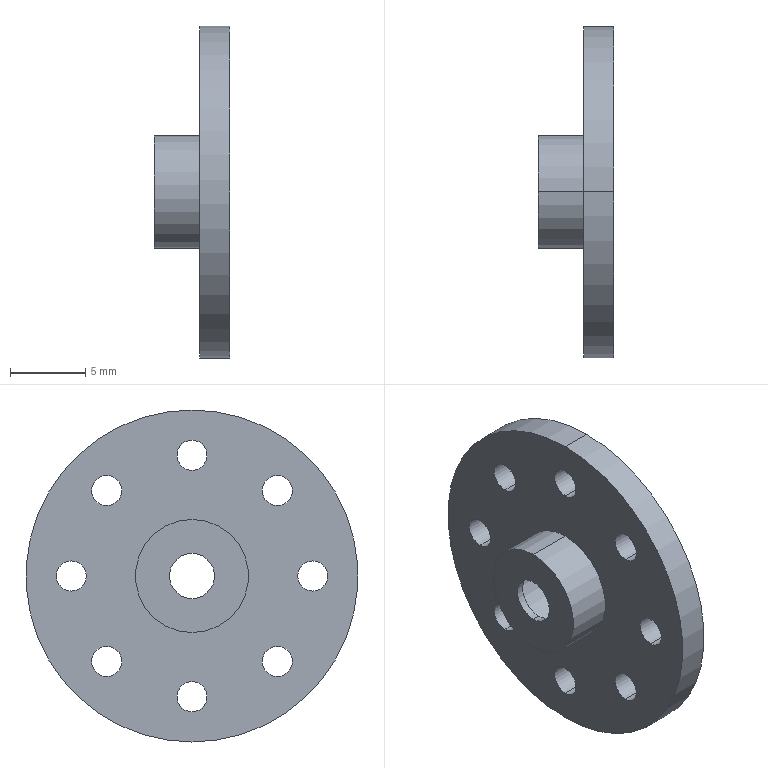Part | SolidWorks | features BaseBody 1 | 1 solid | 28 faces | box 5 x 22 x 22 mm | volume 711.767 mm3 | cylinder 24 | plane 4 | commonest cylinder face diameters 2 x16 3 x2 6 x2 7.5 x2 22 x2
STEP:
#1=CARTESIAN_POINT('',(1.,5.657,4.657));
#2=VERTEX_POINT('',#1);
#3=CARTESIAN_POINT('',(1.,5.657,6.657));
#4=VERTEX_POINT('',#3);
#5=CARTESIAN_POINT('',(1.,5.657,5.657));
#6=DIRECTION('',(-1.,0.,0.));
#7=DIRECTION('',(0.,-0.7071,0.7071));
#8=AXIS2_PLACEMENT_3D('',#5,#6,#7);
#9=CIRCLE('',#8,1.);
#10=EDGE_CURVE('',#2,#4,#9,.T.);
#11=ORIENTED_EDGE('',*,*,#10,.F.);
#12=CARTESIAN_POINT('',(-1.,5.657,4.657));
#13=VERTEX_POINT('',#12);
#14=CARTESIAN_POINT('',(1.,5.657,4.657));
#15=DIRECTION('',(-1.,0.,0.));
#16=VECTOR('',#15,1000.);
#17=LINE('',#14,#16);
#18=EDGE_CURVE('',#2,#13,#17,.T.);
#19=ORIENTED_EDGE('',*,*,#18,.T.);
#20=CARTESIAN_POINT('',(-1.,5.657,6.657));
#21=VERTEX_POINT('',#20);
#22=CARTESIAN_POINT('',(-1.,5.657,5.657));
#23=DIRECTION('',(-1.,0.,0.));
#24=DIRECTION('',(0.,-0.7071,0.7071));
#25=AXIS2_PLACEMENT_3D('',#22,#23,#24);
#26=CIRCLE('',#25,1.);
#27=EDGE_CURVE('',#13,#21,#26,.T.);
#28=ORIENTED_EDGE('',*,*,#27,.T.);
#29=CARTESIAN_POINT('',(1.,5.657,6.657));
#30=DIRECTION('',(-1.,0.,0.));
#31=VECTOR('',#30,1000.);
#32=LINE('',#29,#31);
#33=EDGE_CURVE('',#4,#21,#32,.T.);
#34=ORIENTED_EDGE('',*,*,#33,.F.);
#35=EDGE_LOOP('',(#11,#19,#28,#34));
#36=FACE_OUTER_BOUND('',#35,.T.);
#37=CARTESIAN_POINT('',(1.,5.657,5.657));
#38=DIRECTION('',(-1.,0.,0.));
#39=DIRECTION('',(0.,0.,1.));
#40=AXIS2_PLACEMENT_3D('',#37,#38,#39);
#41=CYLINDRICAL_SURFACE('',#40,1.);
#42=ADVANCED_FACE('',(#36),#41,.F.);
#43=CARTESIAN_POINT('',(1.,0.,7.));
#44=VERTEX_POINT('',#43);
#45=CARTESIAN_POINT('',(1.,0.,9.));
#46=VERTEX_POINT('',#45);
#47=CARTESIAN_POINT('',(1.,0.,8.));
#48=DIRECTION('',(-1.,0.,0.));
#49=DIRECTION('',(0.,-1.,0.));
#50=AXIS2_PLACEMENT_3D('',#47,#48,#49);
#51=CIRCLE('',#50,1.);
#52=EDGE_CURVE('',#44,#46,#51,.T.);
#53=ORIENTED_EDGE('',*,*,#52,.F.);
#54=CARTESIAN_POINT('',(-1.,0.,7.));
#55=VERTEX_POINT('',#54);
#56=CARTESIAN_POINT('',(1.,0.,7.));
#57=DIRECTION('',(-1.,0.,0.));
#58=VECTOR('',#57,1000.);
#59=LINE('',#56,#58);
#60=EDGE_CURVE('',#44,#55,#59,.T.);
#61=ORIENTED_EDGE('',*,*,#60,.T.);
#62=CARTESIAN_POINT('',(-1.,0.,9.));
#63=VERTEX_POINT('',#62);
#64=CARTESIAN_POINT('',(-1.,0.,8.));
#65=DIRECTION('',(-1.,0.,0.));
#66=DIRECTION('',(0.,-1.,0.));
#67=AXIS2_PLACEMENT_3D('',#64,#65,#66);
#68=CIRCLE('',#67,1.);
#69=EDGE_CURVE('',#55,#63,#68,.T.);
#70=ORIENTED_EDGE('',*,*,#69,.T.);
#71=CARTESIAN_POINT('',(1.,0.,9.));
#72=DIRECTION('',(-1.,0.,0.));
#73=VECTOR('',#72,1000.);
#74=LINE('',#71,#73);
#75=EDGE_CURVE('',#46,#63,#74,.T.);
#76=ORIENTED_EDGE('',*,*,#75,.F.);
#77=EDGE_LOOP('',(#53,#61,#70,#76));
#78=FACE_OUTER_BOUND('',#77,.T.);
#79=CARTESIAN_POINT('',(1.,0.,8.));
#80=DIRECTION('',(-1.,0.,0.));
#81=DIRECTION('',(0.,0.,1.));
#82=AXIS2_PLACEMENT_3D('',#79,#80,#81);
#83=CYLINDRICAL_SURFACE('',#82,1.);
#84=ADVANCED_FACE('',(#78),#83,.F.);
#85=CARTESIAN_POINT('',(1.,-5.657,4.657));
#86=VERTEX_POINT('',#85);
#87=CARTESIAN_POINT('',(1.,-5.657,6.657));
#88=VERTEX_POINT('',#87);
#89=CARTESIAN_POINT('',(1.,-5.657,5.657));
#90=DIRECTION('',(-1.,0.,0.));
#91=DIRECTION('',(0.,-0.7071,-0.7071));
#92=AXIS2_PLACEMENT_3D('',#89,#90,#91);
#93=CIRCLE('',#92,1.);
#94=EDGE_CURVE('',#86,#88,#93,.T.);
#95=ORIENTED_EDGE('',*,*,#94,.F.);
#96=CARTESIAN_POINT('',(-1.,-5.657,4.657));
#97=VERTEX_POINT('',#96);
#98=CARTESIAN_POINT('',(1.,-5.657,4.657));
#99=DIRECTION('',(-1.,0.,0.));
#100=VECTOR('',#99,1000.);
#101=LINE('',#98,#100);
#102=EDGE_CURVE('',#86,#97,#101,.T.);
#103=ORIENTED_EDGE('',*,*,#102,.T.);
#104=CARTESIAN_POINT('',(-1.,-5.657,6.657));
#105=VERTEX_POINT('',#104);
#106=CARTESIAN_POINT('',(-1.,-5.657,5.657));
#107=DIRECTION('',(-1.,0.,0.));
#108=DIRECTION('',(0.,-0.7071,-0.7071));
#109=AXIS2_PLACEMENT_3D('',#106,#107,#108);
#110=CIRCLE('',#109,1.);
#111=EDGE_CURVE('',#97,#105,#110,.T.);
#112=ORIENTED_EDGE('',*,*,#111,.T.);
#113=CARTESIAN_POINT('',(1.,-5.657,6.657));
#114=DIRECTION('',(-1.,0.,0.));
#115=VECTOR('',#114,1000.);
#116=LINE('',#113,#115);
#117=EDGE_CURVE('',#88,#105,#116,.T.);
#118=ORIENTED_EDGE('',*,*,#117,.F.);
#119=EDGE_LOOP('',(#95,#103,#112,#118));
#120=FACE_OUTER_BOUND('',#119,.T.);
#121=CARTESIAN_POINT('',(1.,-5.657,5.657));
#122=DIRECTION('',(-1.,0.,0.));
#123=DIRECTION('',(0.,0.,1.));
#124=AXIS2_PLACEMENT_3D('',#121,#122,#123);
#125=CYLINDRICAL_SURFACE('',#124,1.);
#126=ADVANCED_FACE('',(#120),#125,.F.);
#127=CARTESIAN_POINT('',(1.,-8.,-1.));
#128=VERTEX_POINT('',#127);
#129=CARTESIAN_POINT('',(1.,-8.,1.));
#130=VERTEX_POINT('',#129);
#131=CARTESIAN_POINT('',(1.,-8.,0.));
#132=DIRECTION('',(-1.,0.,0.));
#133=DIRECTION('',(0.,0.,-1.));
#134=AXIS2_PLACEMENT_3D('',#131,#132,#133);
#135=CIRCLE('',#134,1.);
#136=EDGE_CURVE('',#128,#130,#135,.T.);
#137=ORIENTED_EDGE('',*,*,#136,.F.);
#138=CARTESIAN_POINT('',(-1.,-8.,-1.));
#139=VERTEX_POINT('',#138);
#140=CARTESIAN_POINT('',(1.,-8.,-1.));
#141=DIRECTION('',(-1.,0.,0.));
#142=VECTOR('',#141,1000.);
#143=LINE('',#140,#142);
#144=EDGE_CURVE('',#128,#139,#143,.T.);
#145=ORIENTED_EDGE('',*,*,#144,.T.);
#146=CARTESIAN_POINT('',(-1.,-8.,1.));
#147=VERTEX_POINT('',#146);
#148=CARTESIAN_POINT('',(-1.,-8.,0.));
#149=DIRECTION('',(-1.,0.,0.));
#150=DIRECTION('',(0.,0.,-1.));
#151=AXIS2_PLACEMENT_3D('',#148,#149,#150);
#152=CIRCLE('',#151,1.);
#153=EDGE_CURVE('',#139,#147,#152,.T.);
#154=ORIENTED_EDGE('',*,*,#153,.T.);
#155=CARTESIAN_POINT('',(1.,-8.,1.));
#156=DIRECTION('',(-1.,0.,0.));
#157=VECTOR('',#156,1000.);
#158=LINE('',#155,#157);
#159=EDGE_CURVE('',#130,#147,#158,.T.);
#160=ORIENTED_EDGE('',*,*,#159,.F.);
#161=EDGE_LOOP('',(#137,#145,#154,#160));
#162=FACE_OUTER_BOUND('',#161,.T.);
#163=CARTESIAN_POINT('',(1.,-8.,0.));
#164=DIRECTION('',(-1.,0.,0.));
#165=DIRECTION('',(0.,0.,1.));
#166=AXIS2_PLACEMENT_3D('',#163,#164,#165);
#167=CYLINDRICAL_SURFACE('',#166,1.);
#168=ADVANCED_FACE('',(#162),#167,.F.);
#169=CARTESIAN_POINT('',(1.,-5.657,-6.657));
#170=VERTEX_POINT('',#169);
#171=CARTESIAN_POINT('',(1.,-5.657,-4.657));
#172=VERTEX_POINT('',#171);
#173=CARTESIAN_POINT('',(1.,-5.657,-5.657));
#174=DIRECTION('',(-1.,0.,0.));
#175=DIRECTION('',(0.,0.7071,-0.7071));
#176=AXIS2_PLACEMENT_3D('',#173,#174,#175);
#177=CIRCLE('',#176,1.);
#178=EDGE_CURVE('',#170,#172,#177,.T.);
#179=ORIENTED_EDGE('',*,*,#178,.F.);
#180=CARTESIAN_POINT('',(-1.,-5.657,-6.657));
#181=VERTEX_POINT('',#180);
#182=CARTESIAN_POINT('',(1.,-5.657,-6.657));
#183=DIRECTION('',(-1.,0.,0.));
#184=VECTOR('',#183,1000.);
#185=LINE('',#182,#184);
#186=EDGE_CURVE('',#170,#181,#185,.T.);
#187=ORIENTED_EDGE('',*,*,#186,.T.);
#188=CARTESIAN_POINT('',(-1.,-5.657,-4.657));
#189=VERTEX_POINT('',#188);
#190=CARTESIAN_POINT('',(-1.,-5.657,-5.657));
#191=DIRECTION('',(-1.,0.,0.));
#192=DIRECTION('',(0.,0.7071,-0.7071));
#193=AXIS2_PLACEMENT_3D('',#190,#191,#192);
#194=CIRCLE('',#193,1.);
#195=EDGE_CURVE('',#181,#189,#194,.T.);
#196=ORIENTED_EDGE('',*,*,#195,.T.);
#197=CARTESIAN_POINT('',(1.,-5.657,-4.657));
#198=DIRECTION('',(-1.,0.,0.));
#199=VECTOR('',#198,1000.);
#200=LINE('',#197,#199);
#201=EDGE_CURVE('',#172,#189,#200,.T.);
#202=ORIENTED_EDGE('',*,*,#201,.F.);
#203=EDGE_LOOP('',(#179,#187,#196,#202));
#204=FACE_OUTER_BOUND('',#203,.T.);
#205=CARTESIAN_POINT('',(1.,-5.657,-5.657));
#206=DIRECTION('',(-1.,0.,0.));
#207=DIRECTION('',(0.,0.,1.));
#208=AXIS2_PLACEMENT_3D('',#205,#206,#207);
#209=CYLINDRICAL_SURFACE('',#208,1.);
#210=ADVANCED_FACE('',(#204),#209,.F.);
#211=CARTESIAN_POINT('',(1.,0.,-9.));
#212=VERTEX_POINT('',#211);
#213=CARTESIAN_POINT('',(1.,0.,-7.));
#214=VERTEX_POINT('',#213);
#215=CARTESIAN_POINT('',(1.,0.,-8.));
#216=DIRECTION('',(-1.,0.,0.));
#217=DIRECTION('',(0.,1.,0.));
#218=AXIS2_PLACEMENT_3D('',#215,#216,#217);
#219=CIRCLE('',#218,1.);
#220=EDGE_CURVE('',#212,#214,#219,.T.);
#221=ORIENTED_EDGE('',*,*,#220,.F.);
#222=CARTESIAN_POINT('',(-1.,0.,-9.));
#223=VERTEX_POINT('',#222);
#224=CARTESIAN_POINT('',(1.,0.,-9.));
#225=DIRECTION('',(-1.,0.,0.));
#226=VECTOR('',#225,1000.);
#227=LINE('',#224,#226);
#228=EDGE_CURVE('',#212,#223,#227,.T.);
#229=ORIENTED_EDGE('',*,*,#228,.T.);
#230=CARTESIAN_POINT('',(-1.,0.,-7.));
#231=VERTEX_POINT('',#230);
#232=CARTESIAN_POINT('',(-1.,0.,-8.));
#233=DIRECTION('',(-1.,0.,0.));
#234=DIRECTION('',(0.,1.,0.));
#235=AXIS2_PLACEMENT_3D('',#232,#233,#234);
#236=CIRCLE('',#235,1.);
#237=EDGE_CURVE('',#223,#231,#236,.T.);
#238=ORIENTED_EDGE('',*,*,#237,.T.);
#239=CARTESIAN_POINT('',(1.,0.,-7.));
#240=DIRECTION('',(-1.,0.,0.));
#241=VECTOR('',#240,1000.);
#242=LINE('',#239,#241);
#243=EDGE_CURVE('',#214,#231,#242,.T.);
#244=ORIENTED_EDGE('',*,*,#243,.F.);
#245=EDGE_LOOP('',(#221,#229,#238,#244));
#246=FACE_OUTER_BOUND('',#245,.T.);
#247=CARTESIAN_POINT('',(1.,0.,-8.));
#248=DIRECTION('',(-1.,0.,0.));
#249=DIRECTION('',(0.,0.,1.));
#250=AXIS2_PLACEMENT_3D('',#247,#248,#249);
#251=CYLINDRICAL_SURFACE('',#250,1.);
#252=ADVANCED_FACE('',(#246),#251,.F.);
#253=CARTESIAN_POINT('',(1.,5.657,-6.657));
#254=VERTEX_POINT('',#253);
#255=CARTESIAN_POINT('',(1.,5.657,-4.657));
#256=VERTEX_POINT('',#255);
#257=CARTESIAN_POINT('',(1.,5.657,-5.657));
#258=DIRECTION('',(-1.,0.,0.));
#259=DIRECTION('',(0.,0.7071,0.7071));
#260=AXIS2_PLACEMENT_3D('',#257,#258,#259);
#261=CIRCLE('',#260,1.);
#262=EDGE_CURVE('',#254,#256,#261,.T.);
#263=ORIENTED_EDGE('',*,*,#262,.F.);
#264=CARTESIAN_POINT('',(-1.,5.657,-6.657));
#265=VERTEX_POINT('',#264);
#266=CARTESIAN_POINT('',(1.,5.657,-6.657));
#267=DIRECTION('',(-1.,0.,0.));
#268=VECTOR('',#267,1000.);
#269=LINE('',#266,#268);
#270=EDGE_CURVE('',#254,#265,#269,.T.);
#271=ORIENTED_EDGE('',*,*,#270,.T.);
#272=CARTESIAN_POINT('',(-1.,5.657,-4.657));
#273=VERTEX_POINT('',#272);
#274=CARTESIAN_POINT('',(-1.,5.657,-5.657));
#275=DIRECTION('',(-1.,0.,0.));
#276=DIRECTION('',(0.,0.7071,0.7071));
#277=AXIS2_PLACEMENT_3D('',#274,#275,#276);
#278=CIRCLE('',#277,1.);
#279=EDGE_CURVE('',#265,#273,#278,.T.);
#280=ORIENTED_EDGE('',*,*,#279,.T.);
#281=CARTESIAN_POINT('',(1.,5.657,-4.657));
#282=DIRECTION('',(-1.,0.,0.));
#283=VECTOR('',#282,1000.);
#284=LINE('',#281,#283);
#285=EDGE_CURVE('',#256,#273,#284,.T.);
#286=ORIENTED_EDGE('',*,*,#285,.F.);
#287=EDGE_LOOP('',(#263,#271,#280,#286));
#288=FACE_OUTER_BOUND('',#287,.T.);
#289=CARTESIAN_POINT('',(1.,5.657,-5.657));
#290=DIRECTION('',(-1.,0.,0.));
#291=DIRECTION('',(0.,0.,1.));
#292=AXIS2_PLACEMENT_3D('',#289,#290,#291);
#293=CYLINDRICAL_SURFACE('',#292,1.);
#294=ADVANCED_FACE('',(#288),#293,.F.);
#295=CARTESIAN_POINT('',(1.,8.,-1.));
#296=VERTEX_POINT('',#295);
#297=CARTESIAN_POINT('',(1.,8.,1.));
#298=VERTEX_POINT('',#297);
#299=CARTESIAN_POINT('',(1.,8.,0.));
#300=DIRECTION('',(-1.,0.,0.));
#301=DIRECTION('',(0.,0.,1.));
#302=AXIS2_PLACEMENT_3D('',#299,#300,#301);
#303=CIRCLE('',#302,1.);
#304=EDGE_CURVE('',#296,#298,#303,.T.);
#305=ORIENTED_EDGE('',*,*,#304,.F.);
#306=CARTESIAN_POINT('',(-1.,8.,-1.));
#307=VERTEX_POINT('',#306);
#308=CARTESIAN_POINT('',(1.,8.,-1.));
#309=DIRECTION('',(-1.,0.,0.));
#310=VECTOR('',#309,1000.);
#311=LINE('',#308,#310);
#312=EDGE_CURVE('',#296,#307,#311,.T.);
#313=ORIENTED_EDGE('',*,*,#312,.T.);
#314=CARTESIAN_POINT('',(-1.,8.,1.));
#315=VERTEX_POINT('',#314);
#316=CARTESIAN_POINT('',(-1.,8.,0.));
#317=DIRECTION('',(-1.,0.,0.));
#318=DIRECTION('',(0.,0.,1.));
#319=AXIS2_PLACEMENT_3D('',#316,#317,#318);
#320=CIRCLE('',#319,1.);
#321=EDGE_CURVE('',#307,#315,#320,.T.);
#322=ORIENTED_EDGE('',*,*,#321,.T.);
#323=CARTESIAN_POINT('',(1.,8.,1.));
#324=DIRECTION('',(-1.,0.,0.));
#325=VECTOR('',#324,1000.);
#326=LINE('',#323,#325);
#327=EDGE_CURVE('',#298,#315,#326,.T.);
#328=ORIENTED_EDGE('',*,*,#327,.F.);
#329=EDGE_LOOP('',(#305,#313,#322,#328));
#330=FACE_OUTER_BOUND('',#329,.T.);
#331=CARTESIAN_POINT('',(1.,8.,0.));
#332=DIRECTION('',(-1.,0.,0.));
#333=DIRECTION('',(0.,0.,1.));
#334=AXIS2_PLACEMENT_3D('',#331,#332,#333);
#335=CYLINDRICAL_SURFACE('',#334,1.);
#336=ADVANCED_FACE('',(#330),#335,.F.);
#337=CARTESIAN_POINT('',(1.,0.,-3.));
#338=VERTEX_POINT('',#337);
#339=CARTESIAN_POINT('',(1.,0.,3.));
#340=VERTEX_POINT('',#339);
#341=CARTESIAN_POINT('',(1.,0.,0.));
#342=DIRECTION('',(-1.,0.,0.));
#343=DIRECTION('',(0.,0.,1.));
#344=AXIS2_PLACEMENT_3D('',#341,#342,#343);
#345=CIRCLE('',#344,3.);
#346=EDGE_CURVE('',#338,#340,#345,.T.);
#347=ORIENTED_EDGE('',*,*,#346,.F.);
#348=CARTESIAN_POINT('',(-3.5,0.,-3.));
#349=VERTEX_POINT('',#348);
#350=CARTESIAN_POINT('',(0.,0.,-3.));
#351=DIRECTION('',(-1.,0.,0.));
#352=VECTOR('',#351,1000.);
#353=LINE('',#350,#352);
#354=EDGE_CURVE('',#338,#349,#353,.T.);
#355=ORIENTED_EDGE('',*,*,#354,.T.);
#356=CARTESIAN_POINT('',(-3.5,0.,3.));
#357=VERTEX_POINT('',#356);
#358=CARTESIAN_POINT('',(-3.5,0.,0.));
#359=DIRECTION('',(-1.,0.,0.));
#360=DIRECTION('',(0.,0.,1.));
#361=AXIS2_PLACEMENT_3D('',#358,#359,#360);
#362=CIRCLE('',#361,3.);
#363=EDGE_CURVE('',#349,#357,#362,.T.);
#364=ORIENTED_EDGE('',*,*,#363,.T.);
#365=CARTESIAN_POINT('',(0.,0.,3.));
#366=DIRECTION('',(-1.,0.,0.));
#367=VECTOR('',#366,1000.);
#368=LINE('',#365,#367);
#369=EDGE_CURVE('',#340,#357,#368,.T.);
#370=ORIENTED_EDGE('',*,*,#369,.F.);
#371=EDGE_LOOP('',(#347,#355,#364,#370));
#372=FACE_OUTER_BOUND('',#371,.T.);
#373=CARTESIAN_POINT('',(0.,0.,0.));
#374=DIRECTION('',(-1.,0.,0.));
#375=DIRECTION('',(0.,0.,1.));
#376=AXIS2_PLACEMENT_3D('',#373,#374,#375);
#377=CYLINDRICAL_SURFACE('',#376,3.);
#378=ADVANCED_FACE('',(#372),#377,.F.);
#379=CARTESIAN_POINT('',(-3.5,0.,-1.5));
#380=VERTEX_POINT('',#379);
#381=CARTESIAN_POINT('',(-3.5,0.,1.5));
#382=VERTEX_POINT('',#381);
#383=CARTESIAN_POINT('',(-3.5,0.,0.));
#384=DIRECTION('',(-1.,0.,0.));
#385=DIRECTION('',(0.,0.,1.));
#386=AXIS2_PLACEMENT_3D('',#383,#384,#385);
#387=CIRCLE('',#386,1.5);
#388=EDGE_CURVE('',#380,#382,#387,.T.);
#389=ORIENTED_EDGE('',*,*,#388,.F.);
#390=CARTESIAN_POINT('',(-4.,0.,-1.5));
#391=VERTEX_POINT('',#390);
#392=CARTESIAN_POINT('',(0.,0.,-1.5));
#393=DIRECTION('',(-1.,0.,0.));
#394=VECTOR('',#393,1000.);
#395=LINE('',#392,#394);
#396=EDGE_CURVE('',#380,#391,#395,.T.);
#397=ORIENTED_EDGE('',*,*,#396,.T.);
#398=CARTESIAN_POINT('',(-4.,0.,1.5));
#399=VERTEX_POINT('',#398);
#400=CARTESIAN_POINT('',(-4.,0.,0.));
#401=DIRECTION('',(-1.,0.,0.));
#402=DIRECTION('',(0.,0.,1.));
#403=AXIS2_PLACEMENT_3D('',#400,#401,#402);
#404=CIRCLE('',#403,1.5);
#405=EDGE_CURVE('',#391,#399,#404,.T.);
#406=ORIENTED_EDGE('',*,*,#405,.T.);
#407=CARTESIAN_POINT('',(0.,0.,1.5));
#408=DIRECTION('',(-1.,0.,0.));
#409=VECTOR('',#408,1000.);
#410=LINE('',#407,#409);
#411=EDGE_CURVE('',#382,#399,#410,.T.);
#412=ORIENTED_EDGE('',*,*,#411,.F.);
#413=EDGE_LOOP('',(#389,#397,#406,#412));
#414=FACE_OUTER_BOUND('',#413,.T.);
#415=CARTESIAN_POINT('',(0.,0.,0.));
#416=DIRECTION('',(-1.,0.,0.));
#417=DIRECTION('',(0.,0.,1.));
#418=AXIS2_PLACEMENT_3D('',#415,#416,#417);
#419=CYLINDRICAL_SURFACE('',#418,1.5);
#420=ADVANCED_FACE('',(#414),#419,.F.);
#421=CARTESIAN_POINT('',(-1.,0.,3.75));
#422=VERTEX_POINT('',#421);
#423=CARTESIAN_POINT('',(-1.,0.,-3.75));
#424=VERTEX_POINT('',#423);
#425=CARTESIAN_POINT('',(-1.,0.,0.));
#426=DIRECTION('',(-1.,0.,0.));
#427=DIRECTION('',(0.,0.,1.));
#428=AXIS2_PLACEMENT_3D('',#425,#426,#427);
#429=CIRCLE('',#428,3.75);
#430=EDGE_CURVE('',#422,#424,#429,.T.);
#431=ORIENTED_EDGE('',*,*,#430,.T.);
#432=CARTESIAN_POINT('',(-4.,0.,-3.75));
#433=VERTEX_POINT('',#432);
#434=CARTESIAN_POINT('',(0.,0.,-3.75));
#435=DIRECTION('',(-1.,0.,0.));
#436=VECTOR('',#435,1000.);
#437=LINE('',#434,#436);
#438=EDGE_CURVE('',#424,#433,#437,.T.);
#439=ORIENTED_EDGE('',*,*,#438,.T.);
#440=CARTESIAN_POINT('',(-4.,0.,3.75));
#441=VERTEX_POINT('',#440);
#442=CARTESIAN_POINT('',(-4.,0.,0.));
#443=DIRECTION('',(-1.,0.,0.));
#444=DIRECTION('',(0.,0.,1.));
#445=AXIS2_PLACEMENT_3D('',#442,#443,#444);
#446=CIRCLE('',#445,3.75);
#447=EDGE_CURVE('',#441,#433,#446,.T.);
#448=ORIENTED_EDGE('',*,*,#447,.F.);
#449=CARTESIAN_POINT('',(0.,0.,3.75));
#450=DIRECTION('',(-1.,0.,0.));
#451=VECTOR('',#450,1000.);
#452=LINE('',#449,#451);
#453=EDGE_CURVE('',#422,#441,#452,.T.);
#454=ORIENTED_EDGE('',*,*,#453,.F.);
#455=EDGE_LOOP('',(#431,#439,#448,#454));
#456=FACE_OUTER_BOUND('',#455,.T.);
#457=CARTESIAN_POINT('',(0.,0.,0.));
#458=DIRECTION('',(-1.,0.,0.));
#459=DIRECTION('',(0.,0.,1.));
#460=AXIS2_PLACEMENT_3D('',#457,#458,#459);
#461=CYLINDRICAL_SURFACE('',#460,3.75);
#462=ADVANCED_FACE('',(#456),#461,.T.);
#463=CARTESIAN_POINT('',(1.,0.,11.));
#464=VERTEX_POINT('',#463);
#465=CARTESIAN_POINT('',(1.,0.,-11.));
#466=VERTEX_POINT('',#465);
#467=CARTESIAN_POINT('',(1.,0.,0.));
#468=DIRECTION('',(-1.,0.,0.));
#469=DIRECTION('',(0.,0.,1.));
#470=AXIS2_PLACEMENT_3D('',#467,#468,#469);
#471=CIRCLE('',#470,11.);
#472=EDGE_CURVE('',#464,#466,#471,.T.);
#473=ORIENTED_EDGE('',*,*,#472,.T.);
#474=CARTESIAN_POINT('',(-1.,0.,-11.));
#475=VERTEX_POINT('',#474);
#476=CARTESIAN_POINT('',(0.,0.,-11.));
#477=DIRECTION('',(-1.,0.,0.));
#478=VECTOR('',#477,1000.);
#479=LINE('',#476,#478);
#480=EDGE_CURVE('',#466,#475,#479,.T.);
#481=ORIENTED_EDGE('',*,*,#480,.T.);
#482=CARTESIAN_POINT('',(-1.,0.,11.));
#483=VERTEX_POINT('',#482);
#484=CARTESIAN_POINT('',(-1.,0.,0.));
#485=DIRECTION('',(-1.,0.,0.));
#486=DIRECTION('',(0.,0.,1.));
#487=AXIS2_PLACEMENT_3D('',#484,#485,#486);
#488=CIRCLE('',#487,11.);
#489=EDGE_CURVE('',#483,#475,#488,.T.);
#490=ORIENTED_EDGE('',*,*,#489,.F.);
#491=CARTESIAN_POINT('',(0.,0.,11.));
#492=DIRECTION('',(-1.,0.,0.));
#493=VECTOR('',#492,1000.);
#494=LINE('',#491,#493);
#495=EDGE_CURVE('',#464,#483,#494,.T.);
#496=ORIENTED_EDGE('',*,*,#495,.F.);
#497=EDGE_LOOP('',(#473,#481,#490,#496));
#498=FACE_OUTER_BOUND('',#497,.T.);
#499=CARTESIAN_POINT('',(0.,0.,0.));
#500=DIRECTION('',(-1.,0.,0.));
#501=DIRECTION('',(0.,0.,1.));
#502=AXIS2_PLACEMENT_3D('',#499,#500,#501);
#503=CYLINDRICAL_SURFACE('',#502,11.);
#504=ADVANCED_FACE('',(#498),#503,.T.);
#505=CARTESIAN_POINT('',(1.,5.657,5.657));
#506=DIRECTION('',(-1.,0.,0.));
#507=DIRECTION('',(0.,-0.7071,0.7071));
#508=AXIS2_PLACEMENT_3D('',#505,#506,#507);
#509=CIRCLE('',#508,1.);
#510=EDGE_CURVE('',#4,#2,#509,.T.);
#511=ORIENTED_EDGE('',*,*,#510,.T.);
#512=ORIENTED_EDGE('',*,*,#10,.T.);
#513=EDGE_LOOP('',(#511,#512));
#514=FACE_BOUND('',#513,.T.);
#515=CARTESIAN_POINT('',(1.,0.,8.));
#516=DIRECTION('',(-1.,0.,0.));
#517=DIRECTION('',(0.,-1.,0.));
#518=AXIS2_PLACEMENT_3D('',#515,#516,#517);
#519=CIRCLE('',#518,1.);
#520=EDGE_CURVE('',#46,#44,#519,.T.);
#521=ORIENTED_EDGE('',*,*,#520,.T.);
#522=ORIENTED_EDGE('',*,*,#52,.T.);
#523=EDGE_LOOP('',(#521,#522));
#524=FACE_BOUND('',#523,.T.);
#525=CARTESIAN_POINT('',(1.,-5.657,5.657));
#526=DIRECTION('',(-1.,0.,0.));
#527=DIRECTION('',(0.,-0.7071,-0.7071));
#528=AXIS2_PLACEMENT_3D('',#525,#526,#527);
#529=CIRCLE('',#528,1.);
#530=EDGE_CURVE('',#88,#86,#529,.T.);
#531=ORIENTED_EDGE('',*,*,#530,.T.);
#532=ORIENTED_EDGE('',*,*,#94,.T.);
#533=EDGE_LOOP('',(#531,#532));
#534=FACE_BOUND('',#533,.T.);
#535=CARTESIAN_POINT('',(1.,-8.,0.));
#536=DIRECTION('',(-1.,0.,0.));
#537=DIRECTION('',(0.,0.,-1.));
#538=AXIS2_PLACEMENT_3D('',#535,#536,#537);
#539=CIRCLE('',#538,1.);
#540=EDGE_CURVE('',#130,#128,#539,.T.);
#541=ORIENTED_EDGE('',*,*,#540,.T.);
#542=ORIENTED_EDGE('',*,*,#136,.T.);
#543=EDGE_LOOP('',(#541,#542));
#544=FACE_BOUND('',#543,.T.);
#545=CARTESIAN_POINT('',(1.,-5.657,-5.657));
#546=DIRECTION('',(-1.,0.,0.));
#547=DIRECTION('',(0.,0.7071,-0.7071));
#548=AXIS2_PLACEMENT_3D('',#545,#546,#547);
#549=CIRCLE('',#548,1.);
#550=EDGE_CURVE('',#172,#170,#549,.T.);
#551=ORIENTED_EDGE('',*,*,#550,.T.);
#552=ORIENTED_EDGE('',*,*,#178,.T.);
#553=EDGE_LOOP('',(#551,#552));
#554=FACE_BOUND('',#553,.T.);
#555=CARTESIAN_POINT('',(1.,0.,-8.));
#556=DIRECTION('',(-1.,0.,0.));
#557=DIRECTION('',(0.,1.,0.));
#558=AXIS2_PLACEMENT_3D('',#555,#556,#557);
#559=CIRCLE('',#558,1.);
#560=EDGE_CURVE('',#214,#212,#559,.T.);
#561=ORIENTED_EDGE('',*,*,#560,.T.);
#562=ORIENTED_EDGE('',*,*,#220,.T.);
#563=EDGE_LOOP('',(#561,#562));
#564=FACE_BOUND('',#563,.T.);
#565=CARTESIAN_POINT('',(1.,5.657,-5.657));
#566=DIRECTION('',(-1.,0.,0.));
#567=DIRECTION('',(0.,0.7071,0.7071));
#568=AXIS2_PLACEMENT_3D('',#565,#566,#567);
#569=CIRCLE('',#568,1.);
#570=EDGE_CURVE('',#256,#254,#569,.T.);
#571=ORIENTED_EDGE('',*,*,#570,.T.);
#572=ORIENTED_EDGE('',*,*,#262,.T.);
#573=EDGE_LOOP('',(#571,#572));
#574=FACE_BOUND('',#573,.T.);
#575=CARTESIAN_POINT('',(1.,8.,0.));
#576=DIRECTION('',(-1.,0.,0.));
#577=DIRECTION('',(0.,0.,1.));
#578=AXIS2_PLACEMENT_3D('',#575,#576,#577);
#579=CIRCLE('',#578,1.);
#580=EDGE_CURVE('',#298,#296,#579,.T.);
#581=ORIENTED_EDGE('',*,*,#580,.T.);
#582=ORIENTED_EDGE('',*,*,#304,.T.);
#583=EDGE_LOOP('',(#581,#582));
#584=FACE_BOUND('',#583,.T.);
#585=ORIENTED_EDGE('',*,*,#472,.F.);
#586=CARTESIAN_POINT('',(1.,0.,0.));
#587=DIRECTION('',(-1.,0.,0.));
#588=DIRECTION('',(0.,0.,1.));
#589=AXIS2_PLACEMENT_3D('',#586,#587,#588);
#590=CIRCLE('',#589,11.);
#591=EDGE_CURVE('',#466,#464,#590,.T.);
#592=ORIENTED_EDGE('',*,*,#591,.F.);
#593=EDGE_LOOP('',(#585,#592));
#594=FACE_OUTER_BOUND('',#593,.T.);
#595=CARTESIAN_POINT('',(1.,0.,0.));
#596=DIRECTION('',(-1.,0.,0.));
#597=DIRECTION('',(0.,0.,1.));
#598=AXIS2_PLACEMENT_3D('',#595,#596,#597);
#599=CIRCLE('',#598,3.);
#600=EDGE_CURVE('',#340,#338,#599,.T.);
#601=ORIENTED_EDGE('',*,*,#600,.T.);
#602=ORIENTED_EDGE('',*,*,#346,.T.);
#603=EDGE_LOOP('',(#601,#602));
#604=FACE_BOUND('',#603,.T.);
#605=CARTESIAN_POINT('',(1.,3.,0.));
#606=DIRECTION('',(-1.,0.,0.));
#607=DIRECTION('',(0.,0.,1.));
#608=AXIS2_PLACEMENT_3D('',#605,#606,#607);
#609=PLANE('',#608);
#610=ADVANCED_FACE('',(#514,#524,#534,#544,#554,#564,#574,#584,#594,#604),#609,.F.);
#611=ORIENTED_EDGE('',*,*,#480,.F.);
#612=ORIENTED_EDGE('',*,*,#591,.T.);
#613=ORIENTED_EDGE('',*,*,#495,.T.);
#614=CARTESIAN_POINT('',(-1.,0.,0.));
#615=DIRECTION('',(-1.,0.,0.));
#616=DIRECTION('',(0.,0.,1.));
#617=AXIS2_PLACEMENT_3D('',#614,#615,#616);
#618=CIRCLE('',#617,11.);
#619=EDGE_CURVE('',#475,#483,#618,.T.);
#620=ORIENTED_EDGE('',*,*,#619,.F.);
#621=EDGE_LOOP('',(#611,#612,#613,#620));
#622=FACE_OUTER_BOUND('',#621,.T.);
#623=CARTESIAN_POINT('',(0.,0.,0.));
#624=DIRECTION('',(-1.,0.,0.));
#625=DIRECTION('',(0.,0.,1.));
#626=AXIS2_PLACEMENT_3D('',#623,#624,#625);
#627=CYLINDRICAL_SURFACE('',#626,11.);
#628=ADVANCED_FACE('',(#622),#627,.T.);
#629=CARTESIAN_POINT('',(-1.,5.657,5.657));
#630=DIRECTION('',(-1.,0.,0.));
#631=DIRECTION('',(0.,-0.7071,0.7071));
#632=AXIS2_PLACEMENT_3D('',#629,#630,#631);
#633=CIRCLE('',#632,1.);
#634=EDGE_CURVE('',#21,#13,#633,.T.);
#635=ORIENTED_EDGE('',*,*,#634,.F.);
#636=ORIENTED_EDGE('',*,*,#27,.F.);
#637=EDGE_LOOP('',(#635,#636));
#638=FACE_BOUND('',#637,.T.);
#639=CARTESIAN_POINT('',(-1.,0.,8.));
#640=DIRECTION('',(-1.,0.,0.));
#641=DIRECTION('',(0.,-1.,0.));
#642=AXIS2_PLACEMENT_3D('',#639,#640,#641);
#643=CIRCLE('',#642,1.);
#644=EDGE_CURVE('',#63,#55,#643,.T.);
#645=ORIENTED_EDGE('',*,*,#644,.F.);
#646=ORIENTED_EDGE('',*,*,#69,.F.);
#647=EDGE_LOOP('',(#645,#646));
#648=FACE_BOUND('',#647,.T.);
#649=CARTESIAN_POINT('',(-1.,-5.657,5.657));
#650=DIRECTION('',(-1.,0.,0.));
#651=DIRECTION('',(0.,-0.7071,-0.7071));
#652=AXIS2_PLACEMENT_3D('',#649,#650,#651);
#653=CIRCLE('',#652,1.);
#654=EDGE_CURVE('',#105,#97,#653,.T.);
#655=ORIENTED_EDGE('',*,*,#654,.F.);
#656=ORIENTED_EDGE('',*,*,#111,.F.);
#657=EDGE_LOOP('',(#655,#656));
#658=FACE_BOUND('',#657,.T.);
#659=CARTESIAN_POINT('',(-1.,-8.,0.));
#660=DIRECTION('',(-1.,0.,0.));
#661=DIRECTION('',(0.,0.,-1.));
#662=AXIS2_PLACEMENT_3D('',#659,#660,#661);
#663=CIRCLE('',#662,1.);
#664=EDGE_CURVE('',#147,#139,#663,.T.);
#665=ORIENTED_EDGE('',*,*,#664,.F.);
#666=ORIENTED_EDGE('',*,*,#153,.F.);
#667=EDGE_LOOP('',(#665,#666));
#668=FACE_BOUND('',#667,.T.);
#669=CARTESIAN_POINT('',(-1.,-5.657,-5.657));
#670=DIRECTION('',(-1.,0.,0.));
#671=DIRECTION('',(0.,0.7071,-0.7071));
#672=AXIS2_PLACEMENT_3D('',#669,#670,#671);
#673=CIRCLE('',#672,1.);
#674=EDGE_CURVE('',#189,#181,#673,.T.);
#675=ORIENTED_EDGE('',*,*,#674,.F.);
#676=ORIENTED_EDGE('',*,*,#195,.F.);
#677=EDGE_LOOP('',(#675,#676));
#678=FACE_BOUND('',#677,.T.);
#679=CARTESIAN_POINT('',(-1.,0.,-8.));
#680=DIRECTION('',(-1.,0.,0.));
#681=DIRECTION('',(0.,1.,0.));
#682=AXIS2_PLACEMENT_3D('',#679,#680,#681);
#683=CIRCLE('',#682,1.);
#684=EDGE_CURVE('',#231,#223,#683,.T.);
#685=ORIENTED_EDGE('',*,*,#684,.F.);
#686=ORIENTED_EDGE('',*,*,#237,.F.);
#687=EDGE_LOOP('',(#685,#686));
#688=FACE_BOUND('',#687,.T.);
#689=CARTESIAN_POINT('',(-1.,5.657,-5.657));
#690=DIRECTION('',(-1.,0.,0.));
#691=DIRECTION('',(0.,0.7071,0.7071));
#692=AXIS2_PLACEMENT_3D('',#689,#690,#691);
#693=CIRCLE('',#692,1.);
#694=EDGE_CURVE('',#273,#265,#693,.T.);
#695=ORIENTED_EDGE('',*,*,#694,.F.);
#696=ORIENTED_EDGE('',*,*,#279,.F.);
#697=EDGE_LOOP('',(#695,#696));
#698=FACE_BOUND('',#697,.T.);
#699=CARTESIAN_POINT('',(-1.,8.,0.));
#700=DIRECTION('',(-1.,0.,0.));
#701=DIRECTION('',(0.,0.,1.));
#702=AXIS2_PLACEMENT_3D('',#699,#700,#701);
#703=CIRCLE('',#702,1.);
#704=EDGE_CURVE('',#315,#307,#703,.T.);
#705=ORIENTED_EDGE('',*,*,#704,.F.);
#706=ORIENTED_EDGE('',*,*,#321,.F.);
#707=EDGE_LOOP('',(#705,#706));
#708=FACE_BOUND('',#707,.T.);
#709=ORIENTED_EDGE('',*,*,#430,.F.);
#710=CARTESIAN_POINT('',(-1.,0.,0.));
#711=DIRECTION('',(-1.,0.,0.));
#712=DIRECTION('',(0.,0.,1.));
#713=AXIS2_PLACEMENT_3D('',#710,#711,#712);
#714=CIRCLE('',#713,3.75);
#715=EDGE_CURVE('',#424,#422,#714,.T.);
#716=ORIENTED_EDGE('',*,*,#715,.F.);
#717=EDGE_LOOP('',(#709,#716));
#718=FACE_BOUND('',#717,.T.);
#719=ORIENTED_EDGE('',*,*,#489,.T.);
#720=ORIENTED_EDGE('',*,*,#619,.T.);
#721=EDGE_LOOP('',(#719,#720));
#722=FACE_OUTER_BOUND('',#721,.T.);
#723=CARTESIAN_POINT('',(-1.,11.,0.));
#724=DIRECTION('',(1.,0.,0.));
#725=DIRECTION('',(0.,0.,-1.));
#726=AXIS2_PLACEMENT_3D('',#723,#724,#725);
#727=PLANE('',#726);
#728=ADVANCED_FACE('',(#638,#648,#658,#668,#678,#688,#698,#708,#718,#722),#727,.F.);
#729=ORIENTED_EDGE('',*,*,#438,.F.);
#730=ORIENTED_EDGE('',*,*,#715,.T.);
#731=ORIENTED_EDGE('',*,*,#453,.T.);
#732=CARTESIAN_POINT('',(-4.,0.,0.));
#733=DIRECTION('',(-1.,0.,0.));
#734=DIRECTION('',(0.,0.,1.));
#735=AXIS2_PLACEMENT_3D('',#732,#733,#734);
#736=CIRCLE('',#735,3.75);
#737=EDGE_CURVE('',#433,#441,#736,.T.);
#738=ORIENTED_EDGE('',*,*,#737,.F.);
#739=EDGE_LOOP('',(#729,#730,#731,#738));
#740=FACE_OUTER_BOUND('',#739,.T.);
#741=CARTESIAN_POINT('',(0.,0.,0.));
#742=DIRECTION('',(-1.,0.,0.));
#743=DIRECTION('',(0.,0.,1.));
#744=AXIS2_PLACEMENT_3D('',#741,#742,#743);
#745=CYLINDRICAL_SURFACE('',#744,3.75);
#746=ADVANCED_FACE('',(#740),#745,.T.);
#747=CARTESIAN_POINT('',(-4.,0.,0.));
#748=DIRECTION('',(-1.,0.,0.));
#749=DIRECTION('',(0.,0.,1.));
#750=AXIS2_PLACEMENT_3D('',#747,#748,#749);
#751=CIRCLE('',#750,1.5);
#752=EDGE_CURVE('',#399,#391,#751,.T.);
#753=ORIENTED_EDGE('',*,*,#752,.F.);
#754=ORIENTED_EDGE('',*,*,#405,.F.);
#755=EDGE_LOOP('',(#753,#754));
#756=FACE_BOUND('',#755,.T.);
#757=ORIENTED_EDGE('',*,*,#447,.T.);
#758=ORIENTED_EDGE('',*,*,#737,.T.);
#759=EDGE_LOOP('',(#757,#758));
#760=FACE_OUTER_BOUND('',#759,.T.);
#761=CARTESIAN_POINT('',(-4.,3.75,0.));
#762=DIRECTION('',(1.,0.,0.));
#763=DIRECTION('',(0.,0.,-1.));
#764=AXIS2_PLACEMENT_3D('',#761,#762,#763);
#765=PLANE('',#764);
#766=ADVANCED_FACE('',(#756,#760),#765,.F.);
#767=ORIENTED_EDGE('',*,*,#396,.F.);
#768=CARTESIAN_POINT('',(-3.5,0.,0.));
#769=DIRECTION('',(-1.,0.,0.));
#770=DIRECTION('',(0.,0.,1.));
#771=AXIS2_PLACEMENT_3D('',#768,#769,#770);
#772=CIRCLE('',#771,1.5);
#773=EDGE_CURVE('',#382,#380,#772,.T.);
#774=ORIENTED_EDGE('',*,*,#773,.F.);
#775=ORIENTED_EDGE('',*,*,#411,.T.);
#776=ORIENTED_EDGE('',*,*,#752,.T.);
#777=EDGE_LOOP('',(#767,#774,#775,#776));
#778=FACE_OUTER_BOUND('',#777,.T.);
#779=CARTESIAN_POINT('',(0.,0.,0.));
#780=DIRECTION('',(-1.,0.,0.));
#781=DIRECTION('',(0.,0.,1.));
#782=AXIS2_PLACEMENT_3D('',#779,#780,#781);
#783=CYLINDRICAL_SURFACE('',#782,1.5);
#784=ADVANCED_FACE('',(#778),#783,.F.);
#785=CARTESIAN_POINT('',(-3.5,0.,0.));
#786=DIRECTION('',(-1.,0.,0.));
#787=DIRECTION('',(0.,0.,1.));
#788=AXIS2_PLACEMENT_3D('',#785,#786,#787);
#789=CIRCLE('',#788,3.);
#790=EDGE_CURVE('',#357,#349,#789,.T.);
#791=ORIENTED_EDGE('',*,*,#790,.F.);
#792=ORIENTED_EDGE('',*,*,#363,.F.);
#793=EDGE_LOOP('',(#791,#792));
#794=FACE_OUTER_BOUND('',#793,.T.);
#795=ORIENTED_EDGE('',*,*,#773,.T.);
#796=ORIENTED_EDGE('',*,*,#388,.T.);
#797=EDGE_LOOP('',(#795,#796));
#798=FACE_BOUND('',#797,.T.);
#799=CARTESIAN_POINT('',(-3.5,3.,0.));
#800=DIRECTION('',(-1.,0.,0.));
#801=DIRECTION('',(0.,0.,1.));
#802=AXIS2_PLACEMENT_3D('',#799,#800,#801);
#803=PLANE('',#802);
#804=ADVANCED_FACE('',(#794,#798),#803,.F.);
#805=ORIENTED_EDGE('',*,*,#354,.F.);
#806=ORIENTED_EDGE('',*,*,#600,.F.);
#807=ORIENTED_EDGE('',*,*,#369,.T.);
#808=ORIENTED_EDGE('',*,*,#790,.T.);
#809=EDGE_LOOP('',(#805,#806,#807,#808));
#810=FACE_OUTER_BOUND('',#809,.T.);
#811=CARTESIAN_POINT('',(0.,0.,0.));
#812=DIRECTION('',(-1.,0.,0.));
#813=DIRECTION('',(0.,0.,1.));
#814=AXIS2_PLACEMENT_3D('',#811,#812,#813);
#815=CYLINDRICAL_SURFACE('',#814,3.);
#816=ADVANCED_FACE('',(#810),#815,.F.);
#817=ORIENTED_EDGE('',*,*,#312,.F.);
#818=ORIENTED_EDGE('',*,*,#580,.F.);
#819=ORIENTED_EDGE('',*,*,#327,.T.);
#820=ORIENTED_EDGE('',*,*,#704,.T.);
#821=EDGE_LOOP('',(#817,#818,#819,#820));
#822=FACE_OUTER_BOUND('',#821,.T.);
#823=CARTESIAN_POINT('',(1.,8.,0.));
#824=DIRECTION('',(-1.,0.,0.));
#825=DIRECTION('',(0.,0.,1.));
#826=AXIS2_PLACEMENT_3D('',#823,#824,#825);
#827=CYLINDRICAL_SURFACE('',#826,1.);
#828=ADVANCED_FACE('',(#822),#827,.F.);
#829=ORIENTED_EDGE('',*,*,#270,.F.);
#830=ORIENTED_EDGE('',*,*,#570,.F.);
#831=ORIENTED_EDGE('',*,*,#285,.T.);
#832=ORIENTED_EDGE('',*,*,#694,.T.);
#833=EDGE_LOOP('',(#829,#830,#831,#832));
#834=FACE_OUTER_BOUND('',#833,.T.);
#835=CARTESIAN_POINT('',(1.,5.657,-5.657));
#836=DIRECTION('',(-1.,0.,0.));
#837=DIRECTION('',(0.,0.,1.));
#838=AXIS2_PLACEMENT_3D('',#835,#836,#837);
#839=CYLINDRICAL_SURFACE('',#838,1.);
#840=ADVANCED_FACE('',(#834),#839,.F.);
#841=ORIENTED_EDGE('',*,*,#228,.F.);
#842=ORIENTED_EDGE('',*,*,#560,.F.);
#843=ORIENTED_EDGE('',*,*,#243,.T.);
#844=ORIENTED_EDGE('',*,*,#684,.T.);
#845=EDGE_LOOP('',(#841,#842,#843,#844));
#846=FACE_OUTER_BOUND('',#845,.T.);
#847=CARTESIAN_POINT('',(1.,0.,-8.));
#848=DIRECTION('',(-1.,0.,0.));
#849=DIRECTION('',(0.,0.,1.));
#850=AXIS2_PLACEMENT_3D('',#847,#848,#849);
#851=CYLINDRICAL_SURFACE('',#850,1.);
#852=ADVANCED_FACE('',(#846),#851,.F.);
#853=ORIENTED_EDGE('',*,*,#186,.F.);
#854=ORIENTED_EDGE('',*,*,#550,.F.);
#855=ORIENTED_EDGE('',*,*,#201,.T.);
#856=ORIENTED_EDGE('',*,*,#674,.T.);
#857=EDGE_LOOP('',(#853,#854,#855,#856));
#858=FACE_OUTER_BOUND('',#857,.T.);
#859=CARTESIAN_POINT('',(1.,-5.657,-5.657));
#860=DIRECTION('',(-1.,0.,0.));
#861=DIRECTION('',(0.,0.,1.));
#862=AXIS2_PLACEMENT_3D('',#859,#860,#861);
#863=CYLINDRICAL_SURFACE('',#862,1.);
#864=ADVANCED_FACE('',(#858),#863,.F.);
#865=ORIENTED_EDGE('',*,*,#144,.F.);
#866=ORIENTED_EDGE('',*,*,#540,.F.);
#867=ORIENTED_EDGE('',*,*,#159,.T.);
#868=ORIENTED_EDGE('',*,*,#664,.T.);
#869=EDGE_LOOP('',(#865,#866,#867,#868));
#870=FACE_OUTER_BOUND('',#869,.T.);
#871=CARTESIAN_POINT('',(1.,-8.,0.));
#872=DIRECTION('',(-1.,0.,0.));
#873=DIRECTION('',(0.,0.,1.));
#874=AXIS2_PLACEMENT_3D('',#871,#872,#873);
#875=CYLINDRICAL_SURFACE('',#874,1.);
#876=ADVANCED_FACE('',(#870),#875,.F.);
#877=ORIENTED_EDGE('',*,*,#102,.F.);
#878=ORIENTED_EDGE('',*,*,#530,.F.);
#879=ORIENTED_EDGE('',*,*,#117,.T.);
#880=ORIENTED_EDGE('',*,*,#654,.T.);
#881=EDGE_LOOP('',(#877,#878,#879,#880));
#882=FACE_OUTER_BOUND('',#881,.T.);
#883=CARTESIAN_POINT('',(1.,-5.657,5.657));
#884=DIRECTION('',(-1.,0.,0.));
#885=DIRECTION('',(0.,0.,1.));
#886=AXIS2_PLACEMENT_3D('',#883,#884,#885);
#887=CYLINDRICAL_SURFACE('',#886,1.);
#888=ADVANCED_FACE('',(#882),#887,.F.);
#889=ORIENTED_EDGE('',*,*,#60,.F.);
#890=ORIENTED_EDGE('',*,*,#520,.F.);
#891=ORIENTED_EDGE('',*,*,#75,.T.);
#892=ORIENTED_EDGE('',*,*,#644,.T.);
#893=EDGE_LOOP('',(#889,#890,#891,#892));
#894=FACE_OUTER_BOUND('',#893,.T.);
#895=CARTESIAN_POINT('',(1.,0.,8.));
#896=DIRECTION('',(-1.,0.,0.));
#897=DIRECTION('',(0.,0.,1.));
#898=AXIS2_PLACEMENT_3D('',#895,#896,#897);
#899=CYLINDRICAL_SURFACE('',#898,1.);
#900=ADVANCED_FACE('',(#894),#899,.F.);
#901=ORIENTED_EDGE('',*,*,#18,.F.);
#902=ORIENTED_EDGE('',*,*,#510,.F.);
#903=ORIENTED_EDGE('',*,*,#33,.T.);
#904=ORIENTED_EDGE('',*,*,#634,.T.);
#905=EDGE_LOOP('',(#901,#902,#903,#904));
#906=FACE_OUTER_BOUND('',#905,.T.);
#907=CARTESIAN_POINT('',(1.,5.657,5.657));
#908=DIRECTION('',(-1.,0.,0.));
#909=DIRECTION('',(0.,0.,1.));
#910=AXIS2_PLACEMENT_3D('',#907,#908,#909);
#911=CYLINDRICAL_SURFACE('',#910,1.);
#912=ADVANCED_FACE('',(#906),#911,.F.);
#913=CLOSED_SHELL('',(#42,#84,#126,#168,#210,#252,#294,#336,#378,#420,#462,#504,#610,#628,#728,#746,#766,#784,#804,#816,#828,#840,#852,#864,#876,#888,#900,#912));
#914=MANIFOLD_SOLID_BREP('',#913);
#915=CARTESIAN_POINT('',(0.,0.,0.));
#916=DIRECTION('',(0.,0.,1.));
#917=DIRECTION('',(1.,0.,0.));
#918=AXIS2_PLACEMENT_3D('',#915,#916,#917);
#919=(LENGTH_UNIT()NAMED_UNIT(*)SI_UNIT(.MILLI.,.METRE.));
#920=UNCERTAINTY_MEASURE_WITH_UNIT(LENGTH_MEASURE(0.00001),#919,'','');
#921=(NAMED_UNIT(*)PLANE_ANGLE_UNIT()SI_UNIT($,.RADIAN.));
#922=(NAMED_UNIT(*)SI_UNIT($,.STERADIAN.)SOLID_ANGLE_UNIT());
#923=(GEOMETRIC_REPRESENTATION_CONTEXT(3)GLOBAL_UNCERTAINTY_ASSIGNED_CONTEXT((#920))GLOBAL_UNIT_ASSIGNED_CONTEXT((#919,#921,#922))REPRESENTATION_CONTEXT('',''));
#924=ADVANCED_BREP_SHAPE_REPRESENTATION('',(#914,#918),#923);